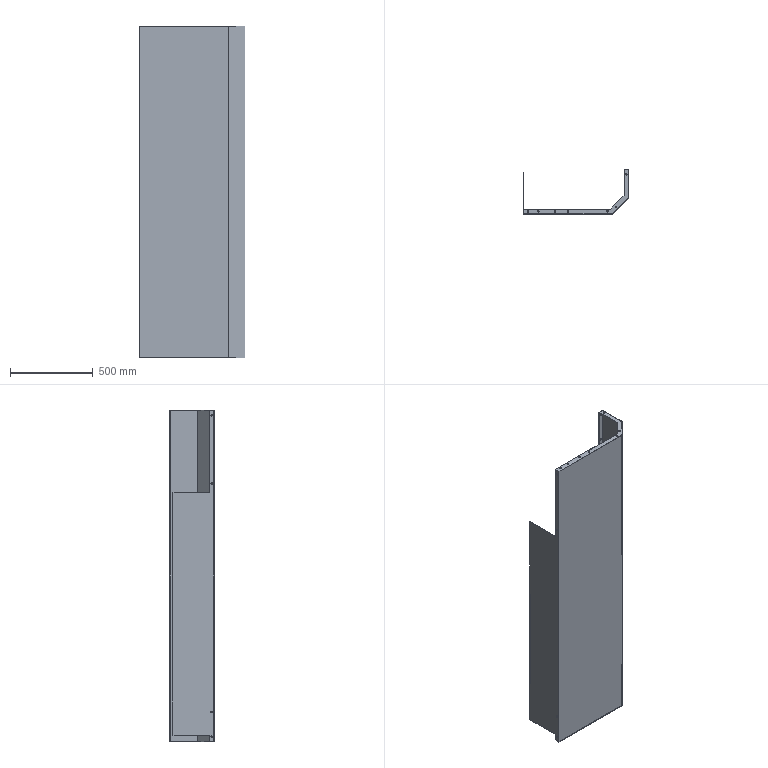Part | SolidWorks | features ICE 11, ExtruThin 1 | 1 solid | 60 faces | box 641 x 270 x 2005 mm | volume 4371242 mm3 | cylinder 38 | plane 22 | commonest cylinder face diameters 9 x38